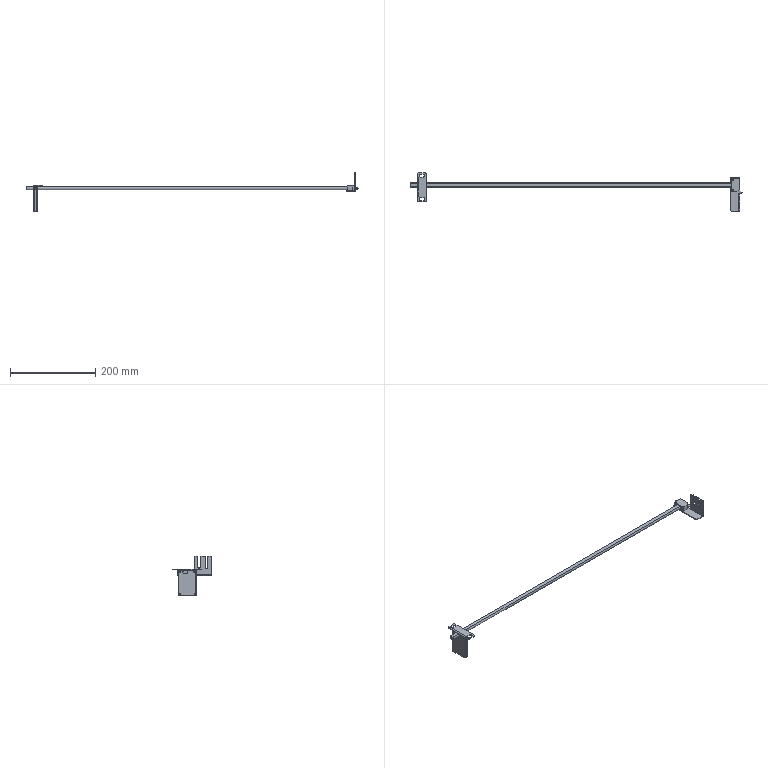Part | SolidWorks | 4 solids | 209 faces | box 779.985 x 90 x 92.8 mm | volume 90208 mm3 | plane 144 | cylinder 65 | commonest cylinder face diameters 4 x14 3.5 x9 2.5 x8 6 x7 2.6 x4 3 x4